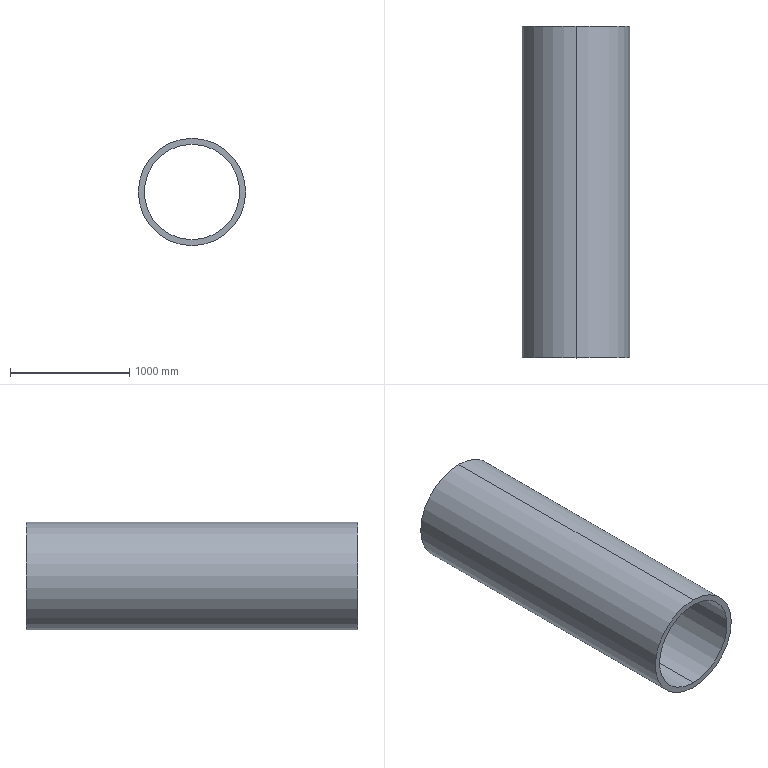Part | SolidWorks | features Extrusion 1, MoveFace 1 | 1 solid | 6 faces | box 900 x 2782 x 900 mm | volume 371446207 mm3 | cylinder 4 | plane 2 | commonest cylinder face diameters 800 x2 900 x2
STEP:
#1=CARTESIAN_POINT('',(0.,1650.,-400.));
#2=VERTEX_POINT('',#1);
#3=CARTESIAN_POINT('',(0.,1650.,400.));
#4=VERTEX_POINT('',#3);
#5=CARTESIAN_POINT('',(0.,1650.,0.));
#6=DIRECTION('',(0.,1.,0.));
#7=DIRECTION('',(0.,0.,1.));
#8=AXIS2_PLACEMENT_3D('',#5,#6,#7);
#9=CIRCLE('',#8,400.);
#10=EDGE_CURVE('',#2,#4,#9,.T.);
#11=ORIENTED_EDGE('',*,*,#10,.T.);
#12=CARTESIAN_POINT('',(0.,-1132.,400.));
#13=VERTEX_POINT('',#12);
#14=CARTESIAN_POINT('',(0.,1650.,400.));
#15=DIRECTION('',(0.,-1.,0.));
#16=VECTOR('',#15,1000.);
#17=LINE('',#14,#16);
#18=EDGE_CURVE('',#4,#13,#17,.T.);
#19=ORIENTED_EDGE('',*,*,#18,.T.);
#20=CARTESIAN_POINT('',(0.,-1132.,-400.));
#21=VERTEX_POINT('',#20);
#22=CARTESIAN_POINT('',(0.,-1132.,0.));
#23=DIRECTION('',(0.,1.,0.));
#24=DIRECTION('',(0.,0.,1.));
#25=AXIS2_PLACEMENT_3D('',#22,#23,#24);
#26=CIRCLE('',#25,400.);
#27=EDGE_CURVE('',#21,#13,#26,.T.);
#28=ORIENTED_EDGE('',*,*,#27,.F.);
#29=CARTESIAN_POINT('',(0.,1650.,-400.));
#30=DIRECTION('',(0.,-1.,0.));
#31=VECTOR('',#30,1000.);
#32=LINE('',#29,#31);
#33=EDGE_CURVE('',#2,#21,#32,.T.);
#34=ORIENTED_EDGE('',*,*,#33,.F.);
#35=EDGE_LOOP('',(#11,#19,#28,#34));
#36=FACE_OUTER_BOUND('',#35,.T.);
#37=CARTESIAN_POINT('',(0.,1650.,0.));
#38=DIRECTION('',(0.,-1.,0.));
#39=DIRECTION('',(0.,0.,-1.));
#40=AXIS2_PLACEMENT_3D('',#37,#38,#39);
#41=CYLINDRICAL_SURFACE('',#40,400.);
#42=ADVANCED_FACE('',(#36),#41,.F.);
#43=CARTESIAN_POINT('',(0.,1650.,450.));
#44=VERTEX_POINT('',#43);
#45=CARTESIAN_POINT('',(0.,1650.,-450.));
#46=VERTEX_POINT('',#45);
#47=CARTESIAN_POINT('',(0.,1650.,0.));
#48=DIRECTION('',(0.,1.,0.));
#49=DIRECTION('',(0.,0.,1.));
#50=AXIS2_PLACEMENT_3D('',#47,#48,#49);
#51=CIRCLE('',#50,450.);
#52=EDGE_CURVE('',#44,#46,#51,.T.);
#53=ORIENTED_EDGE('',*,*,#52,.F.);
#54=CARTESIAN_POINT('',(0.,-1132.,450.));
#55=VERTEX_POINT('',#54);
#56=CARTESIAN_POINT('',(0.,1650.,450.));
#57=DIRECTION('',(0.,-1.,0.));
#58=VECTOR('',#57,1000.);
#59=LINE('',#56,#58);
#60=EDGE_CURVE('',#44,#55,#59,.T.);
#61=ORIENTED_EDGE('',*,*,#60,.T.);
#62=CARTESIAN_POINT('',(0.,-1132.,-450.));
#63=VERTEX_POINT('',#62);
#64=CARTESIAN_POINT('',(0.,-1132.,0.));
#65=DIRECTION('',(0.,1.,0.));
#66=DIRECTION('',(0.,0.,1.));
#67=AXIS2_PLACEMENT_3D('',#64,#65,#66);
#68=CIRCLE('',#67,450.);
#69=EDGE_CURVE('',#55,#63,#68,.T.);
#70=ORIENTED_EDGE('',*,*,#69,.T.);
#71=CARTESIAN_POINT('',(0.,1650.,-450.));
#72=DIRECTION('',(0.,-1.,0.));
#73=VECTOR('',#72,1000.);
#74=LINE('',#71,#73);
#75=EDGE_CURVE('',#46,#63,#74,.T.);
#76=ORIENTED_EDGE('',*,*,#75,.F.);
#77=EDGE_LOOP('',(#53,#61,#70,#76));
#78=FACE_OUTER_BOUND('',#77,.T.);
#79=CARTESIAN_POINT('',(0.,1650.,0.));
#80=DIRECTION('',(0.,-1.,0.));
#81=DIRECTION('',(0.,0.,-1.));
#82=AXIS2_PLACEMENT_3D('',#79,#80,#81);
#83=CYLINDRICAL_SURFACE('',#82,450.);
#84=ADVANCED_FACE('',(#78),#83,.T.);
#85=CARTESIAN_POINT('',(0.,1650.,0.));
#86=DIRECTION('',(0.,1.,0.));
#87=DIRECTION('',(0.,0.,1.));
#88=AXIS2_PLACEMENT_3D('',#85,#86,#87);
#89=CIRCLE('',#88,450.);
#90=EDGE_CURVE('',#46,#44,#89,.T.);
#91=ORIENTED_EDGE('',*,*,#90,.T.);
#92=ORIENTED_EDGE('',*,*,#52,.T.);
#93=EDGE_LOOP('',(#91,#92));
#94=FACE_OUTER_BOUND('',#93,.T.);
#95=ORIENTED_EDGE('',*,*,#10,.F.);
#96=CARTESIAN_POINT('',(0.,1650.,0.));
#97=DIRECTION('',(0.,1.,0.));
#98=DIRECTION('',(0.,0.,1.));
#99=AXIS2_PLACEMENT_3D('',#96,#97,#98);
#100=CIRCLE('',#99,400.);
#101=EDGE_CURVE('',#4,#2,#100,.T.);
#102=ORIENTED_EDGE('',*,*,#101,.F.);
#103=EDGE_LOOP('',(#95,#102));
#104=FACE_BOUND('',#103,.T.);
#105=CARTESIAN_POINT('',(0.,1650.,0.));
#106=DIRECTION('',(0.,1.,0.));
#107=DIRECTION('',(0.,0.,1.));
#108=AXIS2_PLACEMENT_3D('',#105,#106,#107);
#109=PLANE('',#108);
#110=ADVANCED_FACE('',(#94,#104),#109,.T.);
#111=CARTESIAN_POINT('',(0.,-1132.,0.));
#112=DIRECTION('',(0.,1.,0.));
#113=DIRECTION('',(0.,0.,1.));
#114=AXIS2_PLACEMENT_3D('',#111,#112,#113);
#115=CIRCLE('',#114,450.);
#116=EDGE_CURVE('',#63,#55,#115,.T.);
#117=ORIENTED_EDGE('',*,*,#116,.F.);
#118=ORIENTED_EDGE('',*,*,#69,.F.);
#119=EDGE_LOOP('',(#117,#118));
#120=FACE_OUTER_BOUND('',#119,.T.);
#121=ORIENTED_EDGE('',*,*,#27,.T.);
#122=CARTESIAN_POINT('',(0.,-1132.,0.));
#123=DIRECTION('',(0.,1.,0.));
#124=DIRECTION('',(0.,0.,1.));
#125=AXIS2_PLACEMENT_3D('',#122,#123,#124);
#126=CIRCLE('',#125,400.);
#127=EDGE_CURVE('',#13,#21,#126,.T.);
#128=ORIENTED_EDGE('',*,*,#127,.T.);
#129=EDGE_LOOP('',(#121,#128));
#130=FACE_BOUND('',#129,.T.);
#131=CARTESIAN_POINT('',(0.,-1132.,0.));
#132=DIRECTION('',(0.,1.,0.));
#133=DIRECTION('',(0.,0.,1.));
#134=AXIS2_PLACEMENT_3D('',#131,#132,#133);
#135=PLANE('',#134);
#136=ADVANCED_FACE('',(#120,#130),#135,.F.);
#137=ORIENTED_EDGE('',*,*,#60,.F.);
#138=ORIENTED_EDGE('',*,*,#90,.F.);
#139=ORIENTED_EDGE('',*,*,#75,.T.);
#140=ORIENTED_EDGE('',*,*,#116,.T.);
#141=EDGE_LOOP('',(#137,#138,#139,#140));
#142=FACE_OUTER_BOUND('',#141,.T.);
#143=CARTESIAN_POINT('',(0.,1650.,0.));
#144=DIRECTION('',(0.,-1.,0.));
#145=DIRECTION('',(0.,0.,-1.));
#146=AXIS2_PLACEMENT_3D('',#143,#144,#145);
#147=CYLINDRICAL_SURFACE('',#146,450.);
#148=ADVANCED_FACE('',(#142),#147,.T.);
#149=ORIENTED_EDGE('',*,*,#18,.F.);
#150=ORIENTED_EDGE('',*,*,#101,.T.);
#151=ORIENTED_EDGE('',*,*,#33,.T.);
#152=ORIENTED_EDGE('',*,*,#127,.F.);
#153=EDGE_LOOP('',(#149,#150,#151,#152));
#154=FACE_OUTER_BOUND('',#153,.T.);
#155=CARTESIAN_POINT('',(0.,1650.,0.));
#156=DIRECTION('',(0.,-1.,0.));
#157=DIRECTION('',(0.,0.,-1.));
#158=AXIS2_PLACEMENT_3D('',#155,#156,#157);
#159=CYLINDRICAL_SURFACE('',#158,400.);
#160=ADVANCED_FACE('',(#154),#159,.F.);
#161=CLOSED_SHELL('',(#42,#84,#110,#136,#148,#160));
#162=MANIFOLD_SOLID_BREP('',#161);
#163=CARTESIAN_POINT('',(0.,0.,0.));
#164=DIRECTION('',(0.,0.,1.));
#165=DIRECTION('',(1.,0.,0.));
#166=AXIS2_PLACEMENT_3D('',#163,#164,#165);
#167=(LENGTH_UNIT()NAMED_UNIT(*)SI_UNIT(.MILLI.,.METRE.));
#168=UNCERTAINTY_MEASURE_WITH_UNIT(LENGTH_MEASURE(0.00001),#167,'','');
#169=(NAMED_UNIT(*)PLANE_ANGLE_UNIT()SI_UNIT($,.RADIAN.));
#170=(NAMED_UNIT(*)SI_UNIT($,.STERADIAN.)SOLID_ANGLE_UNIT());
#171=(GEOMETRIC_REPRESENTATION_CONTEXT(3)GLOBAL_UNCERTAINTY_ASSIGNED_CONTEXT((#168))GLOBAL_UNIT_ASSIGNED_CONTEXT((#167,#169,#170))REPRESENTATION_CONTEXT('',''));
#172=ADVANCED_BREP_SHAPE_REPRESENTATION('',(#162,#166),#171);